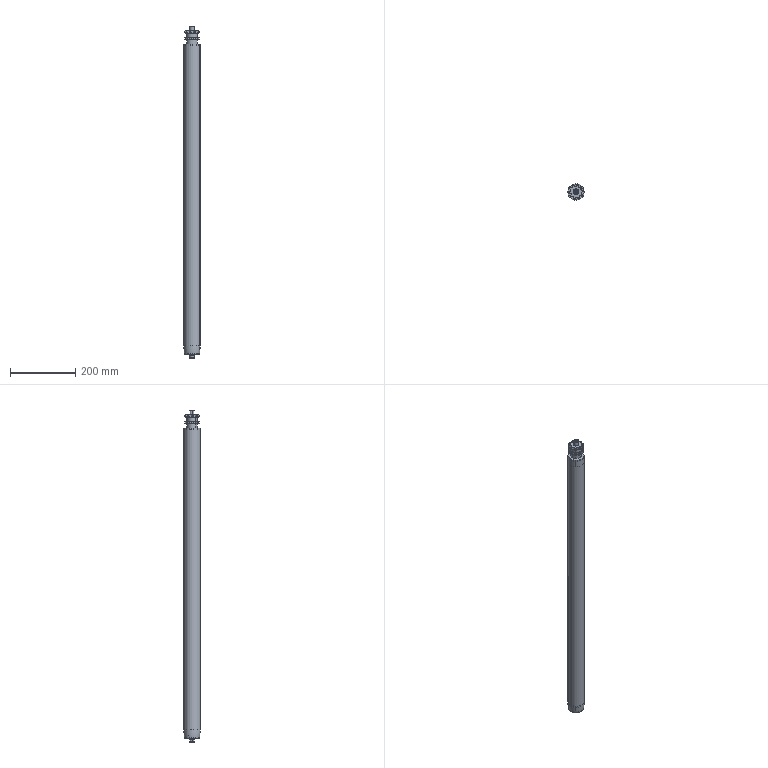Part | SolidWorks | 4 solids | 239 faces | box 50 x 50 x 1020 mm | volume 431386 mm3 | plane 97 | cylinder 74 | cone 52 | torus 16 | commonest cylinder face diameters 46 x22 7.92 x20 6.8 x4 15 x4 32 x4 47.6 x4